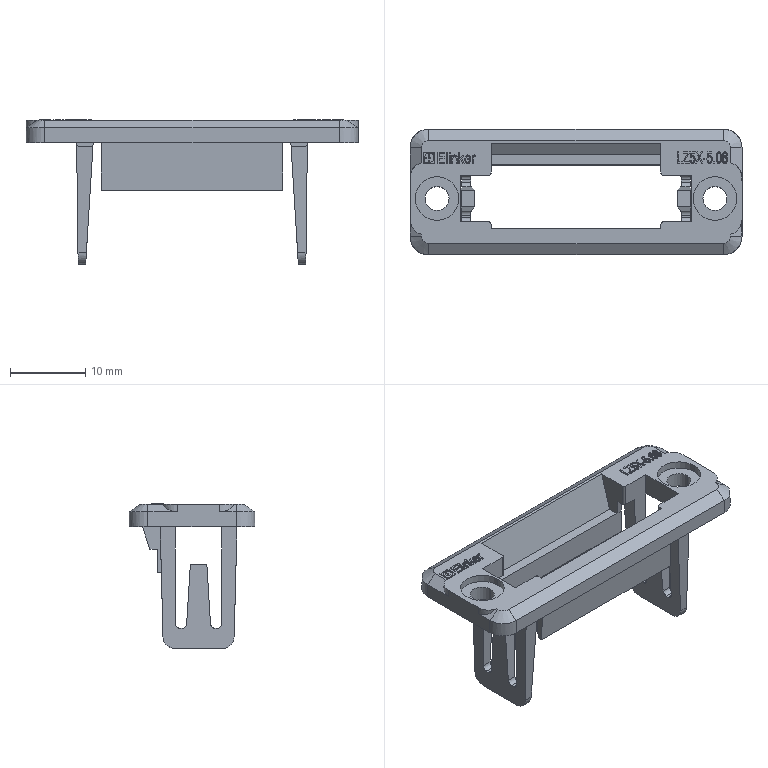Part | NX | features BREP 1 | 1 solid | 1088 faces | box 44.2 x 16.75 x 19.3 mm | volume 1766 mm3 | plane 990 | spline 52 | cylinder 42 | cone 4 | commonest cylinder face diameters 1.2 x8 3.2 x8 0.252 x4 0.6 x4 4.035 x4 5 x4